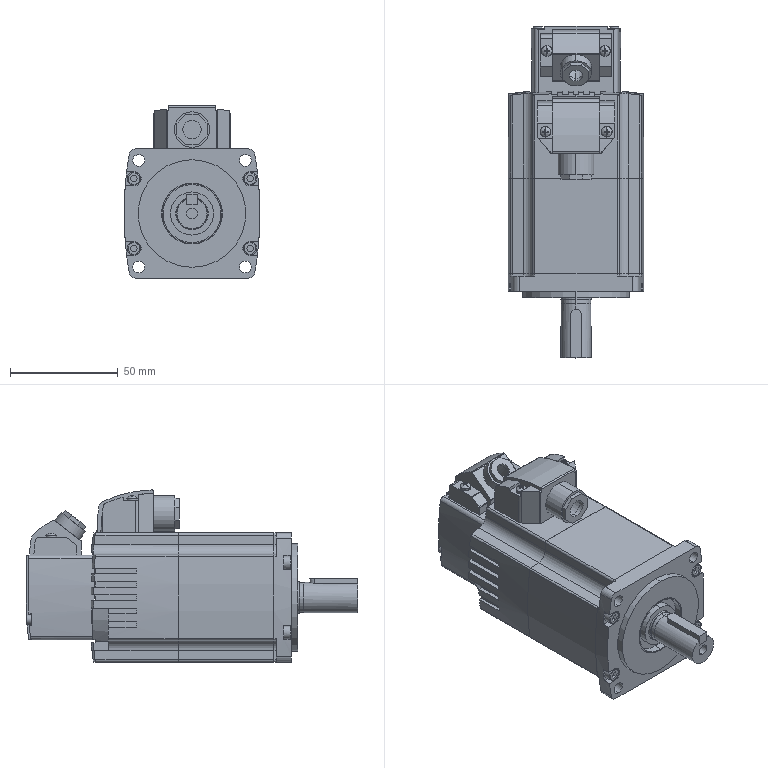Part | STEP file | 8 solids | 742 faces | box 63.062 x 154.188 x 80 mm | volume 326216 mm3 | plane 441 | cylinder 247 | spline 54 | commonest cylinder face diameters 1.2 x24 2 x24 9.4 x12 5 x11 6 x9 2.8 x8